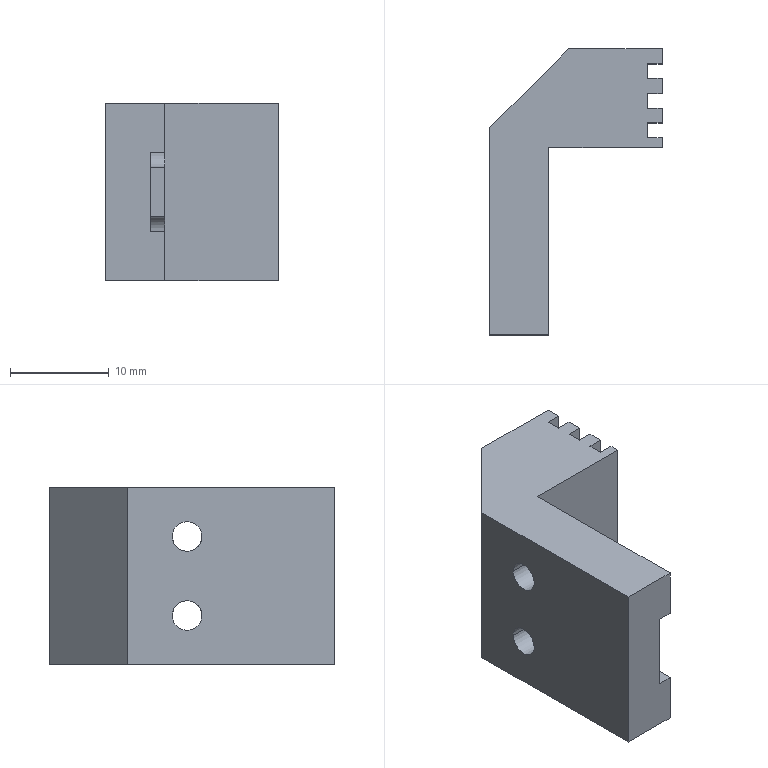Part | SolidWorks | features ICE 3, Chamfer 1, Extrusion 1 | 1 solid | 29 faces | box 17.5 x 29 x 18 mm | volume 4245 mm3 | plane 25 | cylinder 4 | commonest cylinder face diameters 3 x4
STEP:
#1=CARTESIAN_POINT('',(0.,16.5,-4.));
#2=VERTEX_POINT('',#1);
#3=CARTESIAN_POINT('',(0.,13.5,-4.));
#4=VERTEX_POINT('',#3);
#5=CARTESIAN_POINT('',(0.,15.,-4.));
#6=DIRECTION('',(-1.,0.,0.));
#7=DIRECTION('',(0.,0.,-1.));
#8=AXIS2_PLACEMENT_3D('',#5,#6,#7);
#9=CIRCLE('',#8,1.5);
#10=EDGE_CURVE('',#2,#4,#9,.T.);
#11=ORIENTED_EDGE('',*,*,#10,.T.);
#12=CARTESIAN_POINT('',(4.5,13.5,-4.));
#13=VERTEX_POINT('',#12);
#14=CARTESIAN_POINT('',(-0.001,13.5,-4.));
#15=DIRECTION('',(1.,0.,0.));
#16=VECTOR('',#15,1000.);
#17=LINE('',#14,#16);
#18=EDGE_CURVE('',#4,#13,#17,.T.);
#19=ORIENTED_EDGE('',*,*,#18,.T.);
#20=CARTESIAN_POINT('',(6.,13.5,-4.));
#21=VERTEX_POINT('',#20);
#22=CARTESIAN_POINT('',(-0.001,13.5,-4.));
#23=DIRECTION('',(1.,0.,0.));
#24=VECTOR('',#23,1000.);
#25=LINE('',#22,#24);
#26=EDGE_CURVE('',#13,#21,#25,.T.);
#27=ORIENTED_EDGE('',*,*,#26,.T.);
#28=CARTESIAN_POINT('',(6.,16.5,-4.));
#29=VERTEX_POINT('',#28);
#30=CARTESIAN_POINT('',(6.,15.,-4.));
#31=DIRECTION('',(1.,0.,0.));
#32=DIRECTION('',(0.,1.,0.));
#33=AXIS2_PLACEMENT_3D('',#30,#31,#32);
#34=CIRCLE('',#33,1.5);
#35=EDGE_CURVE('',#21,#29,#34,.T.);
#36=ORIENTED_EDGE('',*,*,#35,.T.);
#37=CARTESIAN_POINT('',(-0.001,16.5,-4.));
#38=DIRECTION('',(1.,0.,0.));
#39=VECTOR('',#38,1000.);
#40=LINE('',#37,#39);
#41=EDGE_CURVE('',#2,#29,#40,.T.);
#42=ORIENTED_EDGE('',*,*,#41,.F.);
#43=EDGE_LOOP('',(#11,#19,#27,#36,#42));
#44=FACE_OUTER_BOUND('',#43,.T.);
#45=CARTESIAN_POINT('',(-0.001,15.,-4.));
#46=DIRECTION('',(1.,0.,0.));
#47=DIRECTION('',(0.,1.,0.));
#48=AXIS2_PLACEMENT_3D('',#45,#46,#47);
#49=CYLINDRICAL_SURFACE('',#48,1.5);
#50=ADVANCED_FACE('',(#44),#49,.F.);
#51=CARTESIAN_POINT('',(0.,16.5,4.));
#52=VERTEX_POINT('',#51);
#53=CARTESIAN_POINT('',(0.,13.5,4.));
#54=VERTEX_POINT('',#53);
#55=CARTESIAN_POINT('',(0.,15.,4.));
#56=DIRECTION('',(-1.,0.,0.));
#57=DIRECTION('',(0.,0.,-1.));
#58=AXIS2_PLACEMENT_3D('',#55,#56,#57);
#59=CIRCLE('',#58,1.5);
#60=EDGE_CURVE('',#52,#54,#59,.T.);
#61=ORIENTED_EDGE('',*,*,#60,.T.);
#62=CARTESIAN_POINT('',(4.5,13.5,4.));
#63=VERTEX_POINT('',#62);
#64=CARTESIAN_POINT('',(-0.001,13.5,4.));
#65=DIRECTION('',(1.,0.,0.));
#66=VECTOR('',#65,1000.);
#67=LINE('',#64,#66);
#68=EDGE_CURVE('',#54,#63,#67,.T.);
#69=ORIENTED_EDGE('',*,*,#68,.T.);
#70=CARTESIAN_POINT('',(4.5,15.,2.5));
#71=VERTEX_POINT('',#70);
#72=CARTESIAN_POINT('',(4.5,15.,4.));
#73=DIRECTION('',(-1.,0.,0.));
#74=DIRECTION('',(0.,1.,0.));
#75=AXIS2_PLACEMENT_3D('',#72,#73,#74);
#76=CIRCLE('',#75,1.5);
#77=EDGE_CURVE('',#71,#63,#76,.T.);
#78=ORIENTED_EDGE('',*,*,#77,.F.);
#79=CARTESIAN_POINT('',(6.,15.,2.5));
#80=VERTEX_POINT('',#79);
#81=CARTESIAN_POINT('',(-0.001,15.,2.5));
#82=DIRECTION('',(1.,0.,0.));
#83=VECTOR('',#82,1000.);
#84=LINE('',#81,#83);
#85=EDGE_CURVE('',#71,#80,#84,.T.);
#86=ORIENTED_EDGE('',*,*,#85,.T.);
#87=CARTESIAN_POINT('',(6.,16.5,4.));
#88=VERTEX_POINT('',#87);
#89=CARTESIAN_POINT('',(6.,15.,4.));
#90=DIRECTION('',(1.,0.,0.));
#91=DIRECTION('',(0.,1.,0.));
#92=AXIS2_PLACEMENT_3D('',#89,#90,#91);
#93=CIRCLE('',#92,1.5);
#94=EDGE_CURVE('',#80,#88,#93,.T.);
#95=ORIENTED_EDGE('',*,*,#94,.T.);
#96=CARTESIAN_POINT('',(-0.001,16.5,4.));
#97=DIRECTION('',(1.,0.,0.));
#98=VECTOR('',#97,1000.);
#99=LINE('',#96,#98);
#100=EDGE_CURVE('',#52,#88,#99,.T.);
#101=ORIENTED_EDGE('',*,*,#100,.F.);
#102=EDGE_LOOP('',(#61,#69,#78,#86,#95,#101));
#103=FACE_OUTER_BOUND('',#102,.T.);
#104=CARTESIAN_POINT('',(-0.001,15.,4.));
#105=DIRECTION('',(1.,0.,0.));
#106=DIRECTION('',(0.,1.,0.));
#107=AXIS2_PLACEMENT_3D('',#104,#105,#106);
#108=CYLINDRICAL_SURFACE('',#107,1.5);
#109=ADVANCED_FACE('',(#103),#108,.F.);
#110=CARTESIAN_POINT('',(17.5,27.5,9.));
#111=VERTEX_POINT('',#110);
#112=CARTESIAN_POINT('',(17.5,29.,9.));
#113=VERTEX_POINT('',#112);
#114=CARTESIAN_POINT('',(17.5,29.,9.));
#115=DIRECTION('',(0.,1.,0.));
#116=VECTOR('',#115,1000.);
#117=LINE('',#114,#116);
#118=EDGE_CURVE('',#111,#113,#117,.T.);
#119=ORIENTED_EDGE('',*,*,#118,.F.);
#120=CARTESIAN_POINT('',(17.5,27.5,-9.));
#121=VERTEX_POINT('',#120);
#122=CARTESIAN_POINT('',(17.5,27.5,9.));
#123=DIRECTION('',(0.,0.,1.));
#124=VECTOR('',#123,1000.);
#125=LINE('',#122,#124);
#126=EDGE_CURVE('',#121,#111,#125,.T.);
#127=ORIENTED_EDGE('',*,*,#126,.F.);
#128=CARTESIAN_POINT('',(17.5,29.,-9.));
#129=VERTEX_POINT('',#128);
#130=CARTESIAN_POINT('',(17.5,29.,-9.));
#131=DIRECTION('',(0.,1.,0.));
#132=VECTOR('',#131,1000.);
#133=LINE('',#130,#132);
#134=EDGE_CURVE('',#121,#129,#133,.T.);
#135=ORIENTED_EDGE('',*,*,#134,.T.);
#136=CARTESIAN_POINT('',(17.5,29.,9.));
#137=DIRECTION('',(0.,0.,-1.));
#138=VECTOR('',#137,1000.);
#139=LINE('',#136,#138);
#140=EDGE_CURVE('',#113,#129,#139,.T.);
#141=ORIENTED_EDGE('',*,*,#140,.F.);
#142=EDGE_LOOP('',(#119,#127,#135,#141));
#143=FACE_OUTER_BOUND('',#142,.T.);
#144=CARTESIAN_POINT('',(17.5,29.,9.));
#145=DIRECTION('',(-1.,0.,0.));
#146=DIRECTION('',(0.,0.,1.));
#147=AXIS2_PLACEMENT_3D('',#144,#145,#146);
#148=PLANE('',#147);
#149=ADVANCED_FACE('',(#143),#148,.F.);
#150=CARTESIAN_POINT('',(17.5,24.5,-9.));
#151=VERTEX_POINT('',#150);
#152=CARTESIAN_POINT('',(17.5,26.,-9.));
#153=VERTEX_POINT('',#152);
#154=CARTESIAN_POINT('',(17.5,29.,-9.));
#155=DIRECTION('',(0.,1.,0.));
#156=VECTOR('',#155,1000.);
#157=LINE('',#154,#156);
#158=EDGE_CURVE('',#151,#153,#157,.T.);
#159=ORIENTED_EDGE('',*,*,#158,.T.);
#160=CARTESIAN_POINT('',(17.5,26.,9.));
#161=VERTEX_POINT('',#160);
#162=CARTESIAN_POINT('',(17.5,26.,9.));
#163=DIRECTION('',(0.,0.,-1.));
#164=VECTOR('',#163,1000.);
#165=LINE('',#162,#164);
#166=EDGE_CURVE('',#161,#153,#165,.T.);
#167=ORIENTED_EDGE('',*,*,#166,.F.);
#168=CARTESIAN_POINT('',(17.5,24.5,9.));
#169=VERTEX_POINT('',#168);
#170=CARTESIAN_POINT('',(17.5,29.,9.));
#171=DIRECTION('',(0.,1.,0.));
#172=VECTOR('',#171,1000.);
#173=LINE('',#170,#172);
#174=EDGE_CURVE('',#169,#161,#173,.T.);
#175=ORIENTED_EDGE('',*,*,#174,.F.);
#176=CARTESIAN_POINT('',(17.5,24.5,9.));
#177=DIRECTION('',(0.,0.,1.));
#178=VECTOR('',#177,1000.);
#179=LINE('',#176,#178);
#180=EDGE_CURVE('',#151,#169,#179,.T.);
#181=ORIENTED_EDGE('',*,*,#180,.F.);
#182=EDGE_LOOP('',(#159,#167,#175,#181));
#183=FACE_OUTER_BOUND('',#182,.T.);
#184=CARTESIAN_POINT('',(17.5,29.,9.));
#185=DIRECTION('',(-1.,0.,0.));
#186=DIRECTION('',(0.,0.,1.));
#187=AXIS2_PLACEMENT_3D('',#184,#185,#186);
#188=PLANE('',#187);
#189=ADVANCED_FACE('',(#183),#188,.F.);
#190=CARTESIAN_POINT('',(17.5,21.5,-9.));
#191=VERTEX_POINT('',#190);
#192=CARTESIAN_POINT('',(17.5,23.,-9.));
#193=VERTEX_POINT('',#192);
#194=CARTESIAN_POINT('',(17.5,29.,-9.));
#195=DIRECTION('',(0.,1.,0.));
#196=VECTOR('',#195,1000.);
#197=LINE('',#194,#196);
#198=EDGE_CURVE('',#191,#193,#197,.T.);
#199=ORIENTED_EDGE('',*,*,#198,.T.);
#200=CARTESIAN_POINT('',(17.5,23.,9.));
#201=VERTEX_POINT('',#200);
#202=CARTESIAN_POINT('',(17.5,23.,9.));
#203=DIRECTION('',(0.,0.,-1.));
#204=VECTOR('',#203,1000.);
#205=LINE('',#202,#204);
#206=EDGE_CURVE('',#201,#193,#205,.T.);
#207=ORIENTED_EDGE('',*,*,#206,.F.);
#208=CARTESIAN_POINT('',(17.5,21.5,9.));
#209=VERTEX_POINT('',#208);
#210=CARTESIAN_POINT('',(17.5,29.,9.));
#211=DIRECTION('',(0.,1.,0.));
#212=VECTOR('',#211,1000.);
#213=LINE('',#210,#212);
#214=EDGE_CURVE('',#209,#201,#213,.T.);
#215=ORIENTED_EDGE('',*,*,#214,.F.);
#216=CARTESIAN_POINT('',(17.5,21.5,9.));
#217=DIRECTION('',(0.,0.,1.));
#218=VECTOR('',#217,1000.);
#219=LINE('',#216,#218);
#220=EDGE_CURVE('',#191,#209,#219,.T.);
#221=ORIENTED_EDGE('',*,*,#220,.F.);
#222=EDGE_LOOP('',(#199,#207,#215,#221));
#223=FACE_OUTER_BOUND('',#222,.T.);
#224=CARTESIAN_POINT('',(17.5,29.,9.));
#225=DIRECTION('',(-1.,0.,0.));
#226=DIRECTION('',(0.,0.,1.));
#227=AXIS2_PLACEMENT_3D('',#224,#225,#226);
#228=PLANE('',#227);
#229=ADVANCED_FACE('',(#223),#228,.F.);
#230=CARTESIAN_POINT('',(6.,0.,-4.));
#231=VERTEX_POINT('',#230);
#232=CARTESIAN_POINT('',(6.,0.,-9.));
#233=VERTEX_POINT('',#232);
#234=CARTESIAN_POINT('',(6.,0.,9.));
#235=DIRECTION('',(0.,0.,-1.));
#236=VECTOR('',#235,1000.);
#237=LINE('',#234,#236);
#238=EDGE_CURVE('',#231,#233,#237,.T.);
#239=ORIENTED_EDGE('',*,*,#238,.F.);
#240=CARTESIAN_POINT('',(4.5,0.,-4.));
#241=VERTEX_POINT('',#240);
#242=CARTESIAN_POINT('',(4.5,0.,-4.));
#243=DIRECTION('',(1.,0.,0.));
#244=VECTOR('',#243,1000.);
#245=LINE('',#242,#244);
#246=EDGE_CURVE('',#241,#231,#245,.T.);
#247=ORIENTED_EDGE('',*,*,#246,.F.);
#248=CARTESIAN_POINT('',(4.5,0.,4.));
#249=VERTEX_POINT('',#248);
#250=CARTESIAN_POINT('',(4.5,0.,4.));
#251=DIRECTION('',(0.,0.,-1.));
#252=VECTOR('',#251,1000.);
#253=LINE('',#250,#252);
#254=EDGE_CURVE('',#249,#241,#253,.T.);
#255=ORIENTED_EDGE('',*,*,#254,.F.);
#256=CARTESIAN_POINT('',(6.,0.,4.));
#257=VERTEX_POINT('',#256);
#258=CARTESIAN_POINT('',(4.5,0.,4.));
#259=DIRECTION('',(1.,0.,0.));
#260=VECTOR('',#259,1000.);
#261=LINE('',#258,#260);
#262=EDGE_CURVE('',#249,#257,#261,.T.);
#263=ORIENTED_EDGE('',*,*,#262,.T.);
#264=CARTESIAN_POINT('',(6.,0.,9.));
#265=VERTEX_POINT('',#264);
#266=CARTESIAN_POINT('',(6.,0.,9.));
#267=DIRECTION('',(0.,0.,-1.));
#268=VECTOR('',#267,1000.);
#269=LINE('',#266,#268);
#270=EDGE_CURVE('',#265,#257,#269,.T.);
#271=ORIENTED_EDGE('',*,*,#270,.F.);
#272=CARTESIAN_POINT('',(0.,0.,9.));
#273=VERTEX_POINT('',#272);
#274=CARTESIAN_POINT('',(6.,0.,9.));
#275=DIRECTION('',(1.,0.,0.));
#276=VECTOR('',#275,1000.);
#277=LINE('',#274,#276);
#278=EDGE_CURVE('',#273,#265,#277,.T.);
#279=ORIENTED_EDGE('',*,*,#278,.F.);
#280=CARTESIAN_POINT('',(0.,0.,-9.));
#281=VERTEX_POINT('',#280);
#282=CARTESIAN_POINT('',(0.,0.,9.));
#283=DIRECTION('',(0.,0.,-1.));
#284=VECTOR('',#283,1000.);
#285=LINE('',#282,#284);
#286=EDGE_CURVE('',#273,#281,#285,.T.);
#287=ORIENTED_EDGE('',*,*,#286,.T.);
#288=CARTESIAN_POINT('',(6.,0.,-9.));
#289=DIRECTION('',(1.,0.,0.));
#290=VECTOR('',#289,1000.);
#291=LINE('',#288,#290);
#292=EDGE_CURVE('',#281,#233,#291,.T.);
#293=ORIENTED_EDGE('',*,*,#292,.T.);
#294=EDGE_LOOP('',(#239,#247,#255,#263,#271,#279,#287,#293));
#295=FACE_OUTER_BOUND('',#294,.T.);
#296=CARTESIAN_POINT('',(6.,0.,9.));
#297=DIRECTION('',(0.,1.,0.));
#298=DIRECTION('',(-1.,0.,0.));
#299=AXIS2_PLACEMENT_3D('',#296,#297,#298);
#300=PLANE('',#299);
#301=ADVANCED_FACE('',(#295),#300,.F.);
#302=CARTESIAN_POINT('',(6.,15.,-2.5));
#303=VERTEX_POINT('',#302);
#304=CARTESIAN_POINT('',(6.,15.,4.));
#305=DIRECTION('',(0.,0.,1.));
#306=VECTOR('',#305,1000.);
#307=LINE('',#304,#306);
#308=EDGE_CURVE('',#303,#80,#307,.T.);
#309=ORIENTED_EDGE('',*,*,#308,.F.);
#310=CARTESIAN_POINT('',(6.,15.,-4.));
#311=DIRECTION('',(1.,0.,0.));
#312=DIRECTION('',(0.,1.,0.));
#313=AXIS2_PLACEMENT_3D('',#310,#311,#312);
#314=CIRCLE('',#313,1.5);
#315=EDGE_CURVE('',#29,#303,#314,.T.);
#316=ORIENTED_EDGE('',*,*,#315,.F.);
#317=ORIENTED_EDGE('',*,*,#35,.F.);
#318=CARTESIAN_POINT('',(6.,15.,-4.));
#319=DIRECTION('',(0.,1.,0.));
#320=VECTOR('',#319,1000.);
#321=LINE('',#318,#320);
#322=EDGE_CURVE('',#231,#21,#321,.T.);
#323=ORIENTED_EDGE('',*,*,#322,.F.);
#324=ORIENTED_EDGE('',*,*,#238,.T.);
#325=CARTESIAN_POINT('',(6.,19.,-9.));
#326=VERTEX_POINT('',#325);
#327=CARTESIAN_POINT('',(6.,19.,-9.));
#328=DIRECTION('',(0.,1.,0.));
#329=VECTOR('',#328,1000.);
#330=LINE('',#327,#329);
#331=EDGE_CURVE('',#233,#326,#330,.T.);
#332=ORIENTED_EDGE('',*,*,#331,.T.);
#333=CARTESIAN_POINT('',(6.,19.,9.));
#334=VERTEX_POINT('',#333);
#335=CARTESIAN_POINT('',(6.,19.,9.));
#336=DIRECTION('',(0.,0.,-1.));
#337=VECTOR('',#336,1000.);
#338=LINE('',#335,#337);
#339=EDGE_CURVE('',#334,#326,#338,.T.);
#340=ORIENTED_EDGE('',*,*,#339,.F.);
#341=CARTESIAN_POINT('',(6.,19.,9.));
#342=DIRECTION('',(0.,1.,0.));
#343=VECTOR('',#342,1000.);
#344=LINE('',#341,#343);
#345=EDGE_CURVE('',#265,#334,#344,.T.);
#346=ORIENTED_EDGE('',*,*,#345,.F.);
#347=ORIENTED_EDGE('',*,*,#270,.T.);
#348=CARTESIAN_POINT('',(6.,13.5,4.));
#349=VERTEX_POINT('',#348);
#350=CARTESIAN_POINT('',(6.,15.,4.));
#351=DIRECTION('',(0.,-1.,0.));
#352=VECTOR('',#351,1000.);
#353=LINE('',#350,#352);
#354=EDGE_CURVE('',#349,#257,#353,.T.);
#355=ORIENTED_EDGE('',*,*,#354,.F.);
#356=CARTESIAN_POINT('',(6.,15.,4.));
#357=DIRECTION('',(1.,0.,0.));
#358=DIRECTION('',(0.,1.,0.));
#359=AXIS2_PLACEMENT_3D('',#356,#357,#358);
#360=CIRCLE('',#359,1.5);
#361=EDGE_CURVE('',#88,#349,#360,.T.);
#362=ORIENTED_EDGE('',*,*,#361,.F.);
#363=ORIENTED_EDGE('',*,*,#94,.F.);
#364=EDGE_LOOP('',(#309,#316,#317,#323,#324,#332,#340,#346,#347,#355,#362,#363));
#365=FACE_OUTER_BOUND('',#364,.T.);
#366=CARTESIAN_POINT('',(6.,19.,9.));
#367=DIRECTION('',(-1.,0.,0.));
#368=DIRECTION('',(0.,-1.,0.));
#369=AXIS2_PLACEMENT_3D('',#366,#367,#368);
#370=PLANE('',#369);
#371=ADVANCED_FACE('',(#365),#370,.F.);
#372=CARTESIAN_POINT('',(17.5,19.,-9.));
#373=VERTEX_POINT('',#372);
#374=CARTESIAN_POINT('',(17.5,19.,-9.));
#375=DIRECTION('',(1.,0.,0.));
#376=VECTOR('',#375,1000.);
#377=LINE('',#374,#376);
#378=EDGE_CURVE('',#326,#373,#377,.T.);
#379=ORIENTED_EDGE('',*,*,#378,.T.);
#380=CARTESIAN_POINT('',(17.5,19.,9.));
#381=VERTEX_POINT('',#380);
#382=CARTESIAN_POINT('',(17.5,19.,9.));
#383=DIRECTION('',(0.,0.,-1.));
#384=VECTOR('',#383,1000.);
#385=LINE('',#382,#384);
#386=EDGE_CURVE('',#381,#373,#385,.T.);
#387=ORIENTED_EDGE('',*,*,#386,.F.);
#388=CARTESIAN_POINT('',(17.5,19.,9.));
#389=DIRECTION('',(1.,0.,0.));
#390=VECTOR('',#389,1000.);
#391=LINE('',#388,#390);
#392=EDGE_CURVE('',#334,#381,#391,.T.);
#393=ORIENTED_EDGE('',*,*,#392,.F.);
#394=ORIENTED_EDGE('',*,*,#339,.T.);
#395=EDGE_LOOP('',(#379,#387,#393,#394));
#396=FACE_OUTER_BOUND('',#395,.T.);
#397=CARTESIAN_POINT('',(17.5,19.,9.));
#398=DIRECTION('',(0.,1.,0.));
#399=DIRECTION('',(0.,0.,1.));
#400=AXIS2_PLACEMENT_3D('',#397,#398,#399);
#401=PLANE('',#400);
#402=ADVANCED_FACE('',(#396),#401,.F.);
#403=CARTESIAN_POINT('',(17.5,20.,-9.));
#404=VERTEX_POINT('',#403);
#405=CARTESIAN_POINT('',(17.5,29.,-9.));
#406=DIRECTION('',(0.,1.,0.));
#407=VECTOR('',#406,1000.);
#408=LINE('',#405,#407);
#409=EDGE_CURVE('',#373,#404,#408,.T.);
#410=ORIENTED_EDGE('',*,*,#409,.T.);
#411=CARTESIAN_POINT('',(17.5,20.,9.));
#412=VERTEX_POINT('',#411);
#413=CARTESIAN_POINT('',(17.5,20.,9.));
#414=DIRECTION('',(0.,0.,-1.));
#415=VECTOR('',#414,1000.);
#416=LINE('',#413,#415);
#417=EDGE_CURVE('',#412,#404,#416,.T.);
#418=ORIENTED_EDGE('',*,*,#417,.F.);
#419=CARTESIAN_POINT('',(17.5,29.,9.));
#420=DIRECTION('',(0.,1.,0.));
#421=VECTOR('',#420,1000.);
#422=LINE('',#419,#421);
#423=EDGE_CURVE('',#381,#412,#422,.T.);
#424=ORIENTED_EDGE('',*,*,#423,.F.);
#425=ORIENTED_EDGE('',*,*,#386,.T.);
#426=EDGE_LOOP('',(#410,#418,#424,#425));
#427=FACE_OUTER_BOUND('',#426,.T.);
#428=CARTESIAN_POINT('',(17.5,29.,9.));
#429=DIRECTION('',(-1.,0.,0.));
#430=DIRECTION('',(0.,0.,1.));
#431=AXIS2_PLACEMENT_3D('',#428,#429,#430);
#432=PLANE('',#431);
#433=ADVANCED_FACE('',(#427),#432,.F.);
#434=CARTESIAN_POINT('',(8.,29.,-9.));
#435=VERTEX_POINT('',#434);
#436=CARTESIAN_POINT('',(0.,29.,-9.));
#437=DIRECTION('',(-1.,0.,0.));
#438=VECTOR('',#437,1000.);
#439=LINE('',#436,#438);
#440=EDGE_CURVE('',#129,#435,#439,.T.);
#441=ORIENTED_EDGE('',*,*,#440,.T.);
#442=CARTESIAN_POINT('',(8.,29.,9.));
#443=VERTEX_POINT('',#442);
#444=CARTESIAN_POINT('',(8.,29.,9.));
#445=DIRECTION('',(0.,0.,1.));
#446=VECTOR('',#445,1000.);
#447=LINE('',#444,#446);
#448=EDGE_CURVE('',#435,#443,#447,.T.);
#449=ORIENTED_EDGE('',*,*,#448,.T.);
#450=CARTESIAN_POINT('',(0.,29.,9.));
#451=DIRECTION('',(-1.,0.,0.));
#452=VECTOR('',#451,1000.);
#453=LINE('',#450,#452);
#454=EDGE_CURVE('',#113,#443,#453,.T.);
#455=ORIENTED_EDGE('',*,*,#454,.F.);
#456=ORIENTED_EDGE('',*,*,#140,.T.);
#457=EDGE_LOOP('',(#441,#449,#455,#456));
#458=FACE_OUTER_BOUND('',#457,.T.);
#459=CARTESIAN_POINT('',(0.,29.,9.));
#460=DIRECTION('',(0.,-1.,0.));
#461=DIRECTION('',(0.,0.,-1.));
#462=AXIS2_PLACEMENT_3D('',#459,#460,#461);
#463=PLANE('',#462);
#464=ADVANCED_FACE('',(#458),#463,.F.);
#465=ORIENTED_EDGE('',*,*,#10,.F.);
#466=CARTESIAN_POINT('',(0.,15.,-4.));
#467=DIRECTION('',(-1.,0.,0.));
#468=DIRECTION('',(0.,0.,-1.));
#469=AXIS2_PLACEMENT_3D('',#466,#467,#468);
#470=CIRCLE('',#469,1.5);
#471=EDGE_CURVE('',#4,#2,#470,.T.);
#472=ORIENTED_EDGE('',*,*,#471,.F.);
#473=EDGE_LOOP('',(#465,#472));
#474=FACE_BOUND('',#473,.T.);
#475=ORIENTED_EDGE('',*,*,#60,.F.);
#476=CARTESIAN_POINT('',(0.,15.,4.));
#477=DIRECTION('',(-1.,0.,0.));
#478=DIRECTION('',(0.,0.,-1.));
#479=AXIS2_PLACEMENT_3D('',#476,#477,#478);
#480=CIRCLE('',#479,1.5);
#481=EDGE_CURVE('',#54,#52,#480,.T.);
#482=ORIENTED_EDGE('',*,*,#481,.F.);
#483=EDGE_LOOP('',(#475,#482));
#484=FACE_BOUND('',#483,.T.);
#485=CARTESIAN_POINT('',(0.,21.,9.));
#486=VERTEX_POINT('',#485);
#487=CARTESIAN_POINT('',(0.,0.,9.));
#488=DIRECTION('',(0.,-1.,0.));
#489=VECTOR('',#488,1000.);
#490=LINE('',#487,#489);
#491=EDGE_CURVE('',#486,#273,#490,.T.);
#492=ORIENTED_EDGE('',*,*,#491,.F.);
#493=CARTESIAN_POINT('',(0.,21.,-9.));
#494=VERTEX_POINT('',#493);
#495=CARTESIAN_POINT('',(0.,21.,9.));
#496=DIRECTION('',(0.,0.,-1.));
#497=VECTOR('',#496,1000.);
#498=LINE('',#495,#497);
#499=EDGE_CURVE('',#486,#494,#498,.T.);
#500=ORIENTED_EDGE('',*,*,#499,.T.);
#501=CARTESIAN_POINT('',(0.,0.,-9.));
#502=DIRECTION('',(0.,-1.,0.));
#503=VECTOR('',#502,1000.);
#504=LINE('',#501,#503);
#505=EDGE_CURVE('',#494,#281,#504,.T.);
#506=ORIENTED_EDGE('',*,*,#505,.T.);
#507=ORIENTED_EDGE('',*,*,#286,.F.);
#508=EDGE_LOOP('',(#492,#500,#506,#507));
#509=FACE_OUTER_BOUND('',#508,.T.);
#510=CARTESIAN_POINT('',(0.,0.,9.));
#511=DIRECTION('',(1.,0.,0.));
#512=DIRECTION('',(0.,0.,-1.));
#513=AXIS2_PLACEMENT_3D('',#510,#511,#512);
#514=PLANE('',#513);
#515=ADVANCED_FACE('',(#474,#484,#509),#514,.F.);
#516=ORIENTED_EDGE('',*,*,#454,.T.);
#517=CARTESIAN_POINT('',(0.,21.,9.));
#518=DIRECTION('',(-0.7071,-0.7071,0.));
#519=VECTOR('',#518,1000.);
#520=LINE('',#517,#519);
#521=EDGE_CURVE('',#443,#486,#520,.T.);
#522=ORIENTED_EDGE('',*,*,#521,.T.);
#523=ORIENTED_EDGE('',*,*,#491,.T.);
#524=ORIENTED_EDGE('',*,*,#278,.T.);
#525=ORIENTED_EDGE('',*,*,#345,.T.);
#526=ORIENTED_EDGE('',*,*,#392,.T.);
#527=ORIENTED_EDGE('',*,*,#423,.T.);
#528=CARTESIAN_POINT('',(16.,20.,9.));
#529=VERTEX_POINT('',#528);
#530=CARTESIAN_POINT('',(16.,20.,9.));
#531=DIRECTION('',(1.,0.,0.));
#532=VECTOR('',#531,1000.);
#533=LINE('',#530,#532);
#534=EDGE_CURVE('',#529,#412,#533,.T.);
#535=ORIENTED_EDGE('',*,*,#534,.F.);
#536=CARTESIAN_POINT('',(16.,21.5,9.));
#537=VERTEX_POINT('',#536);
#538=CARTESIAN_POINT('',(16.,20.,9.));
#539=DIRECTION('',(0.,-1.,0.));
#540=VECTOR('',#539,1000.);
#541=LINE('',#538,#540);
#542=EDGE_CURVE('',#537,#529,#541,.T.);
#543=ORIENTED_EDGE('',*,*,#542,.F.);
#544=CARTESIAN_POINT('',(16.,21.5,9.));
#545=DIRECTION('',(1.,0.,0.));
#546=VECTOR('',#545,1000.);
#547=LINE('',#544,#546);
#548=EDGE_CURVE('',#537,#209,#547,.T.);
#549=ORIENTED_EDGE('',*,*,#548,.T.);
#550=ORIENTED_EDGE('',*,*,#214,.T.);
#551=CARTESIAN_POINT('',(16.,23.,9.));
#552=VERTEX_POINT('',#551);
#553=CARTESIAN_POINT('',(16.,23.,9.));
#554=DIRECTION('',(1.,0.,0.));
#555=VECTOR('',#554,1000.);
#556=LINE('',#553,#555);
#557=EDGE_CURVE('',#552,#201,#556,.T.);
#558=ORIENTED_EDGE('',*,*,#557,.F.);
#559=CARTESIAN_POINT('',(16.,24.5,9.));
#560=VERTEX_POINT('',#559);
#561=CARTESIAN_POINT('',(16.,23.,9.));
#562=DIRECTION('',(0.,-1.,0.));
#563=VECTOR('',#562,1000.);
#564=LINE('',#561,#563);
#565=EDGE_CURVE('',#560,#552,#564,.T.);
#566=ORIENTED_EDGE('',*,*,#565,.F.);
#567=CARTESIAN_POINT('',(16.,24.5,9.));
#568=DIRECTION('',(1.,0.,0.));
#569=VECTOR('',#568,1000.);
#570=LINE('',#567,#569);
#571=EDGE_CURVE('',#560,#169,#570,.T.);
#572=ORIENTED_EDGE('',*,*,#571,.T.);
#573=ORIENTED_EDGE('',*,*,#174,.T.);
#574=CARTESIAN_POINT('',(16.,26.,9.));
#575=VERTEX_POINT('',#574);
#576=CARTESIAN_POINT('',(16.,26.,9.));
#577=DIRECTION('',(1.,0.,0.));
#578=VECTOR('',#577,1000.);
#579=LINE('',#576,#578);
#580=EDGE_CURVE('',#575,#161,#579,.T.);
#581=ORIENTED_EDGE('',*,*,#580,.F.);
#582=CARTESIAN_POINT('',(16.,27.5,9.));
#583=VERTEX_POINT('',#582);
#584=CARTESIAN_POINT('',(16.,27.5,9.));
#585=DIRECTION('',(0.,-1.,0.));
#586=VECTOR('',#585,1000.);
#587=LINE('',#584,#586);
#588=EDGE_CURVE('',#583,#575,#587,.T.);
#589=ORIENTED_EDGE('',*,*,#588,.F.);
#590=CARTESIAN_POINT('',(16.,27.5,9.));
#591=DIRECTION('',(1.,0.,0.));
#592=VECTOR('',#591,1000.);
#593=LINE('',#590,#592);
#594=EDGE_CURVE('',#583,#111,#593,.T.);
#595=ORIENTED_EDGE('',*,*,#594,.T.);
#596=ORIENTED_EDGE('',*,*,#118,.T.);
#597=EDGE_LOOP('',(#516,#522,#523,#524,#525,#526,#527,#535,#543,#549,#550,#558,#566,#572,#573,#581,#589,#595,#596));
#598=FACE_OUTER_BOUND('',#597,.T.);
#599=CARTESIAN_POINT('',(0.,0.,9.));
#600=DIRECTION('',(0.,0.,-1.));
#601=DIRECTION('',(-1.,0.,0.));
#602=AXIS2_PLACEMENT_3D('',#599,#600,#601);
#603=PLANE('',#602);
#604=ADVANCED_FACE('',(#598),#603,.F.);
#605=ORIENTED_EDGE('',*,*,#505,.F.);
#606=CARTESIAN_POINT('',(-10.5,10.5,-9.));
#607=DIRECTION('',(0.7071,0.7071,0.));
#608=VECTOR('',#607,1000.);
#609=LINE('',#606,#608);
#610=EDGE_CURVE('',#494,#435,#609,.T.);
#611=ORIENTED_EDGE('',*,*,#610,.T.);
#612=ORIENTED_EDGE('',*,*,#440,.F.);
#613=ORIENTED_EDGE('',*,*,#134,.F.);
#614=CARTESIAN_POINT('',(16.,27.5,-9.));
#615=VERTEX_POINT('',#614);
#616=CARTESIAN_POINT('',(16.,27.5,-9.));
#617=DIRECTION('',(1.,0.,0.));
#618=VECTOR('',#617,1000.);
#619=LINE('',#616,#618);
#620=EDGE_CURVE('',#615,#121,#619,.T.);
#621=ORIENTED_EDGE('',*,*,#620,.F.);
#622=CARTESIAN_POINT('',(16.,26.,-9.));
#623=VERTEX_POINT('',#622);
#624=CARTESIAN_POINT('',(16.,27.5,-9.));
#625=DIRECTION('',(0.,1.,0.));
#626=VECTOR('',#625,1000.);
#627=LINE('',#624,#626);
#628=EDGE_CURVE('',#623,#615,#627,.T.);
#629=ORIENTED_EDGE('',*,*,#628,.F.);
#630=CARTESIAN_POINT('',(16.,26.,-9.));
#631=DIRECTION('',(1.,0.,0.));
#632=VECTOR('',#631,1000.);
#633=LINE('',#630,#632);
#634=EDGE_CURVE('',#623,#153,#633,.T.);
#635=ORIENTED_EDGE('',*,*,#634,.T.);
#636=ORIENTED_EDGE('',*,*,#158,.F.);
#637=CARTESIAN_POINT('',(16.,24.5,-9.));
#638=VERTEX_POINT('',#637);
#639=CARTESIAN_POINT('',(16.,24.5,-9.));
#640=DIRECTION('',(1.,0.,0.));
#641=VECTOR('',#640,1000.);
#642=LINE('',#639,#641);
#643=EDGE_CURVE('',#638,#151,#642,.T.);
#644=ORIENTED_EDGE('',*,*,#643,.F.);
#645=CARTESIAN_POINT('',(16.,23.,-9.));
#646=VERTEX_POINT('',#645);
#647=CARTESIAN_POINT('',(16.,23.,-9.));
#648=DIRECTION('',(0.,1.,0.));
#649=VECTOR('',#648,1000.);
#650=LINE('',#647,#649);
#651=EDGE_CURVE('',#646,#638,#650,.T.);
#652=ORIENTED_EDGE('',*,*,#651,.F.);
#653=CARTESIAN_POINT('',(16.,23.,-9.));
#654=DIRECTION('',(1.,0.,0.));
#655=VECTOR('',#654,1000.);
#656=LINE('',#653,#655);
#657=EDGE_CURVE('',#646,#193,#656,.T.);
#658=ORIENTED_EDGE('',*,*,#657,.T.);
#659=ORIENTED_EDGE('',*,*,#198,.F.);
#660=CARTESIAN_POINT('',(16.,21.5,-9.));
#661=VERTEX_POINT('',#660);
#662=CARTESIAN_POINT('',(16.,21.5,-9.));
#663=DIRECTION('',(1.,0.,0.));
#664=VECTOR('',#663,1000.);
#665=LINE('',#662,#664);
#666=EDGE_CURVE('',#661,#191,#665,.T.);
#667=ORIENTED_EDGE('',*,*,#666,.F.);
#668=CARTESIAN_POINT('',(16.,20.,-9.));
#669=VERTEX_POINT('',#668);
#670=CARTESIAN_POINT('',(16.,20.,-9.));
#671=DIRECTION('',(0.,1.,0.));
#672=VECTOR('',#671,1000.);
#673=LINE('',#670,#672);
#674=EDGE_CURVE('',#669,#661,#673,.T.);
#675=ORIENTED_EDGE('',*,*,#674,.F.);
#676=CARTESIAN_POINT('',(16.,20.,-9.));
#677=DIRECTION('',(1.,0.,0.));
#678=VECTOR('',#677,1000.);
#679=LINE('',#676,#678);
#680=EDGE_CURVE('',#669,#404,#679,.T.);
#681=ORIENTED_EDGE('',*,*,#680,.T.);
#682=ORIENTED_EDGE('',*,*,#409,.F.);
#683=ORIENTED_EDGE('',*,*,#378,.F.);
#684=ORIENTED_EDGE('',*,*,#331,.F.);
#685=ORIENTED_EDGE('',*,*,#292,.F.);
#686=EDGE_LOOP('',(#605,#611,#612,#613,#621,#629,#635,#636,#644,#652,#658,#659,#667,#675,#681,#682,#683,#684,#685));
#687=FACE_OUTER_BOUND('',#686,.T.);
#688=CARTESIAN_POINT('',(0.,0.,-9.));
#689=DIRECTION('',(0.,0.,-1.));
#690=DIRECTION('',(-1.,0.,0.));
#691=AXIS2_PLACEMENT_3D('',#688,#689,#690);
#692=PLANE('',#691);
#693=ADVANCED_FACE('',(#687),#692,.T.);
#694=ORIENTED_EDGE('',*,*,#322,.T.);
#695=ORIENTED_EDGE('',*,*,#26,.F.);
#696=CARTESIAN_POINT('',(4.5,15.,-4.));
#697=DIRECTION('',(0.,1.,0.));
#698=VECTOR('',#697,1000.);
#699=LINE('',#696,#698);
#700=EDGE_CURVE('',#241,#13,#699,.T.);
#701=ORIENTED_EDGE('',*,*,#700,.F.);
#702=ORIENTED_EDGE('',*,*,#246,.T.);
#703=EDGE_LOOP('',(#694,#695,#701,#702));
#704=FACE_OUTER_BOUND('',#703,.T.);
#705=CARTESIAN_POINT('',(4.5,15.,-4.));
#706=DIRECTION('',(0.,0.,-1.));
#707=DIRECTION('',(0.,1.,0.));
#708=AXIS2_PLACEMENT_3D('',#705,#706,#707);
#709=PLANE('',#708);
#710=ADVANCED_FACE('',(#704),#709,.F.);
#711=CARTESIAN_POINT('',(4.5,15.,4.));
#712=DIRECTION('',(0.,-1.,0.));
#713=VECTOR('',#712,1000.);
#714=LINE('',#711,#713);
#715=EDGE_CURVE('',#63,#249,#714,.T.);
#716=ORIENTED_EDGE('',*,*,#715,.F.);
#717=CARTESIAN_POINT('',(-0.001,13.5,4.));
#718=DIRECTION('',(-1.,0.,0.));
#719=VECTOR('',#718,1000.);
#720=LINE('',#717,#719);
#721=EDGE_CURVE('',#349,#63,#720,.T.);
#722=ORIENTED_EDGE('',*,*,#721,.F.);
#723=ORIENTED_EDGE('',*,*,#354,.T.);
#724=ORIENTED_EDGE('',*,*,#262,.F.);
#725=EDGE_LOOP('',(#716,#722,#723,#724));
#726=FACE_OUTER_BOUND('',#725,.T.);
#727=CARTESIAN_POINT('',(4.5,15.,4.));
#728=DIRECTION('',(0.,0.,1.));
#729=DIRECTION('',(0.,-1.,0.));
#730=AXIS2_PLACEMENT_3D('',#727,#728,#729);
#731=PLANE('',#730);
#732=ADVANCED_FACE('',(#726),#731,.F.);
#733=CARTESIAN_POINT('',(4.5,15.,-2.5));
#734=VERTEX_POINT('',#733);
#735=CARTESIAN_POINT('',(4.5,15.,4.));
#736=DIRECTION('',(0.,0.,1.));
#737=VECTOR('',#736,1000.);
#738=LINE('',#735,#737);
#739=EDGE_CURVE('',#734,#71,#738,.T.);
#740=ORIENTED_EDGE('',*,*,#739,.F.);
#741=CARTESIAN_POINT('',(-0.001,15.,-2.5));
#742=DIRECTION('',(-1.,0.,0.));
#743=VECTOR('',#742,1000.);
#744=LINE('',#741,#743);
#745=EDGE_CURVE('',#303,#734,#744,.T.);
#746=ORIENTED_EDGE('',*,*,#745,.F.);
#747=ORIENTED_EDGE('',*,*,#308,.T.);
#748=ORIENTED_EDGE('',*,*,#85,.F.);
#749=EDGE_LOOP('',(#740,#746,#747,#748));
#750=FACE_OUTER_BOUND('',#749,.T.);
#751=CARTESIAN_POINT('',(4.5,15.,4.));
#752=DIRECTION('',(0.,1.,0.));
#753=DIRECTION('',(-1.,0.,0.));
#754=AXIS2_PLACEMENT_3D('',#751,#752,#753);
#755=PLANE('',#754);
#756=ADVANCED_FACE('',(#750),#755,.F.);
#757=CARTESIAN_POINT('',(4.5,15.,-4.));
#758=DIRECTION('',(-1.,0.,0.));
#759=DIRECTION('',(0.,1.,0.));
#760=AXIS2_PLACEMENT_3D('',#757,#758,#759);
#761=CIRCLE('',#760,1.5);
#762=EDGE_CURVE('',#13,#734,#761,.T.);
#763=ORIENTED_EDGE('',*,*,#762,.T.);
#764=ORIENTED_EDGE('',*,*,#739,.T.);
#765=ORIENTED_EDGE('',*,*,#77,.T.);
#766=ORIENTED_EDGE('',*,*,#715,.T.);
#767=ORIENTED_EDGE('',*,*,#254,.T.);
#768=ORIENTED_EDGE('',*,*,#700,.T.);
#769=EDGE_LOOP('',(#763,#764,#765,#766,#767,#768));
#770=FACE_OUTER_BOUND('',#769,.T.);
#771=CARTESIAN_POINT('',(4.5,0.,0.));
#772=DIRECTION('',(1.,0.,0.));
#773=DIRECTION('',(0.,1.,0.));
#774=AXIS2_PLACEMENT_3D('',#771,#772,#773);
#775=PLANE('',#774);
#776=ADVANCED_FACE('',(#770),#775,.T.);
#777=ORIENTED_EDGE('',*,*,#68,.F.);
#778=ORIENTED_EDGE('',*,*,#481,.T.);
#779=ORIENTED_EDGE('',*,*,#100,.T.);
#780=ORIENTED_EDGE('',*,*,#361,.T.);
#781=ORIENTED_EDGE('',*,*,#721,.T.);
#782=EDGE_LOOP('',(#777,#778,#779,#780,#781));
#783=FACE_OUTER_BOUND('',#782,.T.);
#784=CARTESIAN_POINT('',(-0.001,15.,4.));
#785=DIRECTION('',(1.,0.,0.));
#786=DIRECTION('',(0.,1.,0.));
#787=AXIS2_PLACEMENT_3D('',#784,#785,#786);
#788=CYLINDRICAL_SURFACE('',#787,1.5);
#789=ADVANCED_FACE('',(#783),#788,.F.);
#790=ORIENTED_EDGE('',*,*,#18,.F.);
#791=ORIENTED_EDGE('',*,*,#471,.T.);
#792=ORIENTED_EDGE('',*,*,#41,.T.);
#793=ORIENTED_EDGE('',*,*,#315,.T.);
#794=ORIENTED_EDGE('',*,*,#745,.T.);
#795=ORIENTED_EDGE('',*,*,#762,.F.);
#796=EDGE_LOOP('',(#790,#791,#792,#793,#794,#795));
#797=FACE_OUTER_BOUND('',#796,.T.);
#798=CARTESIAN_POINT('',(-0.001,15.,-4.));
#799=DIRECTION('',(1.,0.,0.));
#800=DIRECTION('',(0.,1.,0.));
#801=AXIS2_PLACEMENT_3D('',#798,#799,#800);
#802=CYLINDRICAL_SURFACE('',#801,1.5);
#803=ADVANCED_FACE('',(#797),#802,.F.);
#804=ORIENTED_EDGE('',*,*,#220,.T.);
#805=ORIENTED_EDGE('',*,*,#548,.F.);
#806=CARTESIAN_POINT('',(16.,21.5,9.));
#807=DIRECTION('',(0.,0.,1.));
#808=VECTOR('',#807,1000.);
#809=LINE('',#806,#808);
#810=EDGE_CURVE('',#661,#537,#809,.T.);
#811=ORIENTED_EDGE('',*,*,#810,.F.);
#812=ORIENTED_EDGE('',*,*,#666,.T.);
#813=EDGE_LOOP('',(#804,#805,#811,#812));
#814=FACE_OUTER_BOUND('',#813,.T.);
#815=CARTESIAN_POINT('',(16.,21.5,9.));
#816=DIRECTION('',(0.,1.,0.));
#817=DIRECTION('',(-1.,0.,0.));
#818=AXIS2_PLACEMENT_3D('',#815,#816,#817);
#819=PLANE('',#818);
#820=ADVANCED_FACE('',(#814),#819,.F.);
#821=ORIENTED_EDGE('',*,*,#417,.T.);
#822=ORIENTED_EDGE('',*,*,#680,.F.);
#823=CARTESIAN_POINT('',(16.,20.,9.));
#824=DIRECTION('',(0.,0.,-1.));
#825=VECTOR('',#824,1000.);
#826=LINE('',#823,#825);
#827=EDGE_CURVE('',#529,#669,#826,.T.);
#828=ORIENTED_EDGE('',*,*,#827,.F.);
#829=ORIENTED_EDGE('',*,*,#534,.T.);
#830=EDGE_LOOP('',(#821,#822,#828,#829));
#831=FACE_OUTER_BOUND('',#830,.T.);
#832=CARTESIAN_POINT('',(16.,20.,9.));
#833=DIRECTION('',(0.,-1.,0.));
#834=DIRECTION('',(1.,0.,0.));
#835=AXIS2_PLACEMENT_3D('',#832,#833,#834);
#836=PLANE('',#835);
#837=ADVANCED_FACE('',(#831),#836,.F.);
#838=ORIENTED_EDGE('',*,*,#542,.T.);
#839=ORIENTED_EDGE('',*,*,#827,.T.);
#840=ORIENTED_EDGE('',*,*,#674,.T.);
#841=ORIENTED_EDGE('',*,*,#810,.T.);
#842=EDGE_LOOP('',(#838,#839,#840,#841));
#843=FACE_OUTER_BOUND('',#842,.T.);
#844=CARTESIAN_POINT('',(16.,0.,0.));
#845=DIRECTION('',(-1.,0.,0.));
#846=DIRECTION('',(0.,0.,1.));
#847=AXIS2_PLACEMENT_3D('',#844,#845,#846);
#848=PLANE('',#847);
#849=ADVANCED_FACE('',(#843),#848,.F.);
#850=ORIENTED_EDGE('',*,*,#180,.T.);
#851=ORIENTED_EDGE('',*,*,#571,.F.);
#852=CARTESIAN_POINT('',(16.,24.5,9.));
#853=DIRECTION('',(0.,0.,1.));
#854=VECTOR('',#853,1000.);
#855=LINE('',#852,#854);
#856=EDGE_CURVE('',#638,#560,#855,.T.);
#857=ORIENTED_EDGE('',*,*,#856,.F.);
#858=ORIENTED_EDGE('',*,*,#643,.T.);
#859=EDGE_LOOP('',(#850,#851,#857,#858));
#860=FACE_OUTER_BOUND('',#859,.T.);
#861=CARTESIAN_POINT('',(16.,24.5,9.));
#862=DIRECTION('',(0.,1.,0.));
#863=DIRECTION('',(-1.,0.,0.));
#864=AXIS2_PLACEMENT_3D('',#861,#862,#863);
#865=PLANE('',#864);
#866=ADVANCED_FACE('',(#860),#865,.F.);
#867=ORIENTED_EDGE('',*,*,#206,.T.);
#868=ORIENTED_EDGE('',*,*,#657,.F.);
#869=CARTESIAN_POINT('',(16.,23.,9.));
#870=DIRECTION('',(0.,0.,-1.));
#871=VECTOR('',#870,1000.);
#872=LINE('',#869,#871);
#873=EDGE_CURVE('',#552,#646,#872,.T.);
#874=ORIENTED_EDGE('',*,*,#873,.F.);
#875=ORIENTED_EDGE('',*,*,#557,.T.);
#876=EDGE_LOOP('',(#867,#868,#874,#875));
#877=FACE_OUTER_BOUND('',#876,.T.);
#878=CARTESIAN_POINT('',(16.,23.,9.));
#879=DIRECTION('',(0.,-1.,0.));
#880=DIRECTION('',(1.,0.,0.));
#881=AXIS2_PLACEMENT_3D('',#878,#879,#880);
#882=PLANE('',#881);
#883=ADVANCED_FACE('',(#877),#882,.F.);
#884=ORIENTED_EDGE('',*,*,#565,.T.);
#885=ORIENTED_EDGE('',*,*,#873,.T.);
#886=ORIENTED_EDGE('',*,*,#651,.T.);
#887=ORIENTED_EDGE('',*,*,#856,.T.);
#888=EDGE_LOOP('',(#884,#885,#886,#887));
#889=FACE_OUTER_BOUND('',#888,.T.);
#890=CARTESIAN_POINT('',(16.,0.,0.));
#891=DIRECTION('',(-1.,0.,0.));
#892=DIRECTION('',(0.,-1.,0.));
#893=AXIS2_PLACEMENT_3D('',#890,#891,#892);
#894=PLANE('',#893);
#895=ADVANCED_FACE('',(#889),#894,.F.);
#896=ORIENTED_EDGE('',*,*,#126,.T.);
#897=ORIENTED_EDGE('',*,*,#594,.F.);
#898=CARTESIAN_POINT('',(16.,27.5,9.));
#899=DIRECTION('',(0.,0.,1.));
#900=VECTOR('',#899,1000.);
#901=LINE('',#898,#900);
#902=EDGE_CURVE('',#615,#583,#901,.T.);
#903=ORIENTED_EDGE('',*,*,#902,.F.);
#904=ORIENTED_EDGE('',*,*,#620,.T.);
#905=EDGE_LOOP('',(#896,#897,#903,#904));
#906=FACE_OUTER_BOUND('',#905,.T.);
#907=CARTESIAN_POINT('',(16.,27.5,9.));
#908=DIRECTION('',(0.,1.,0.));
#909=DIRECTION('',(-1.,0.,0.));
#910=AXIS2_PLACEMENT_3D('',#907,#908,#909);
#911=PLANE('',#910);
#912=ADVANCED_FACE('',(#906),#911,.F.);
#913=ORIENTED_EDGE('',*,*,#166,.T.);
#914=ORIENTED_EDGE('',*,*,#634,.F.);
#915=CARTESIAN_POINT('',(16.,26.,9.));
#916=DIRECTION('',(0.,0.,-1.));
#917=VECTOR('',#916,1000.);
#918=LINE('',#915,#917);
#919=EDGE_CURVE('',#575,#623,#918,.T.);
#920=ORIENTED_EDGE('',*,*,#919,.F.);
#921=ORIENTED_EDGE('',*,*,#580,.T.);
#922=EDGE_LOOP('',(#913,#914,#920,#921));
#923=FACE_OUTER_BOUND('',#922,.T.);
#924=CARTESIAN_POINT('',(16.,26.,9.));
#925=DIRECTION('',(0.,-1.,0.));
#926=DIRECTION('',(1.,0.,0.));
#927=AXIS2_PLACEMENT_3D('',#924,#925,#926);
#928=PLANE('',#927);
#929=ADVANCED_FACE('',(#923),#928,.F.);
#930=ORIENTED_EDGE('',*,*,#588,.T.);
#931=ORIENTED_EDGE('',*,*,#919,.T.);
#932=ORIENTED_EDGE('',*,*,#628,.T.);
#933=ORIENTED_EDGE('',*,*,#902,.T.);
#934=EDGE_LOOP('',(#930,#931,#932,#933));
#935=FACE_OUTER_BOUND('',#934,.T.);
#936=CARTESIAN_POINT('',(16.,0.,0.));
#937=DIRECTION('',(1.,0.,0.));
#938=DIRECTION('',(0.,0.,-1.));
#939=AXIS2_PLACEMENT_3D('',#936,#937,#938);
#940=PLANE('',#939);
#941=ADVANCED_FACE('',(#935),#940,.T.);
#942=ORIENTED_EDGE('',*,*,#521,.F.);
#943=ORIENTED_EDGE('',*,*,#448,.F.);
#944=ORIENTED_EDGE('',*,*,#610,.F.);
#945=ORIENTED_EDGE('',*,*,#499,.F.);
#946=EDGE_LOOP('',(#942,#943,#944,#945));
#947=FACE_OUTER_BOUND('',#946,.T.);
#948=CARTESIAN_POINT('',(0.,21.,9.));
#949=DIRECTION('',(0.7071,-0.7071,0.));
#950=DIRECTION('',(0.,0.,-1.));
#951=AXIS2_PLACEMENT_3D('',#948,#949,#950);
#952=PLANE('',#951);
#953=ADVANCED_FACE('',(#947),#952,.F.);
#954=CLOSED_SHELL('',(#50,#109,#149,#189,#229,#301,#371,#402,#433,#464,#515,#604,#693,#710,#732,#756,#776,#789,#803,#820,#837,#849,#866,#883,#895,#912,#929,#941,#953));
#955=MANIFOLD_SOLID_BREP('',#954);
#956=CARTESIAN_POINT('',(0.,0.,0.));
#957=DIRECTION('',(0.,0.,1.));
#958=DIRECTION('',(1.,0.,0.));
#959=AXIS2_PLACEMENT_3D('',#956,#957,#958);
#960=(LENGTH_UNIT()NAMED_UNIT(*)SI_UNIT(.MILLI.,.METRE.));
#961=UNCERTAINTY_MEASURE_WITH_UNIT(LENGTH_MEASURE(0.00001),#960,'','');
#962=(NAMED_UNIT(*)PLANE_ANGLE_UNIT()SI_UNIT($,.RADIAN.));
#963=(NAMED_UNIT(*)SI_UNIT($,.STERADIAN.)SOLID_ANGLE_UNIT());
#964=(GEOMETRIC_REPRESENTATION_CONTEXT(3)GLOBAL_UNCERTAINTY_ASSIGNED_CONTEXT((#961))GLOBAL_UNIT_ASSIGNED_CONTEXT((#960,#962,#963))REPRESENTATION_CONTEXT('',''));
#965=ADVANCED_BREP_SHAPE_REPRESENTATION('',(#955,#959),#964);